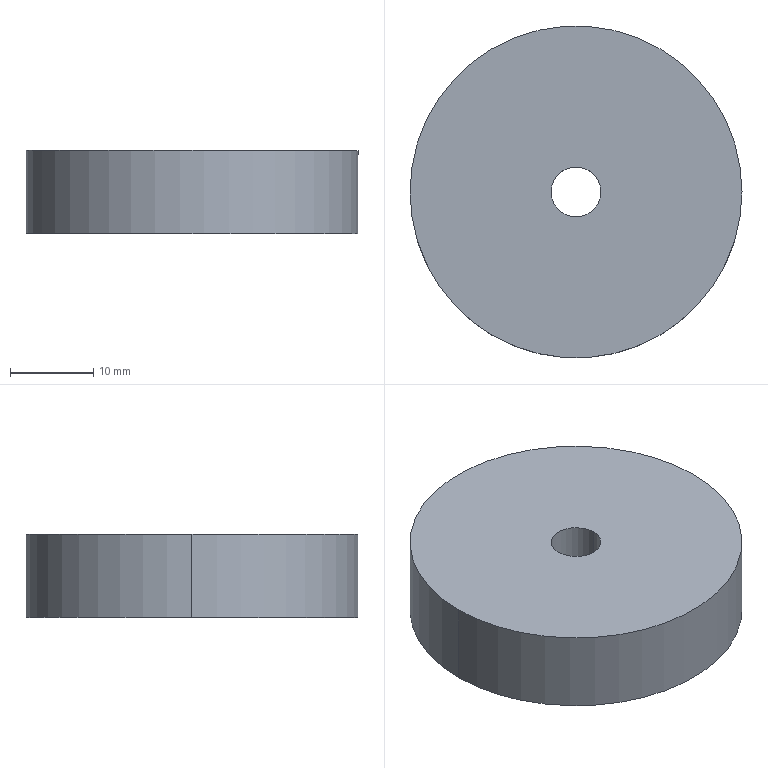Part | SolidWorks | features Revolution 1 | 1 solid | 6 faces | box 40 x 40 x 10 mm | volume 12284 mm3 | cylinder 4 | plane 2 | commonest cylinder face diameters 6 x2 40 x2
STEP:
#1=CARTESIAN_POINT('',(20.,0.,-10.));
#2=VERTEX_POINT('',#1);
#3=CARTESIAN_POINT('',(-20.,0.,-10.));
#4=VERTEX_POINT('',#3);
#5=CARTESIAN_POINT('',(0.,0.,-10.));
#6=DIRECTION('',(0.,0.,1.));
#7=DIRECTION('',(1.,0.,0.));
#8=AXIS2_PLACEMENT_3D('',#5,#6,#7);
#9=CIRCLE('',#8,20.);
#10=EDGE_CURVE('',#2,#4,#9,.T.);
#11=ORIENTED_EDGE('',*,*,#10,.T.);
#12=CARTESIAN_POINT('',(-20.,0.,0.));
#13=VERTEX_POINT('',#12);
#14=CARTESIAN_POINT('',(-20.,0.,129.063));
#15=DIRECTION('',(0.,0.,1.));
#16=VECTOR('',#15,1000.);
#17=LINE('',#14,#16);
#18=EDGE_CURVE('',#4,#13,#17,.T.);
#19=ORIENTED_EDGE('',*,*,#18,.T.);
#20=CARTESIAN_POINT('',(20.,0.,0.));
#21=VERTEX_POINT('',#20);
#22=CARTESIAN_POINT('',(0.,0.,0.));
#23=DIRECTION('',(0.,0.,1.));
#24=DIRECTION('',(1.,0.,0.));
#25=AXIS2_PLACEMENT_3D('',#22,#23,#24);
#26=CIRCLE('',#25,20.);
#27=EDGE_CURVE('',#21,#13,#26,.T.);
#28=ORIENTED_EDGE('',*,*,#27,.F.);
#29=CARTESIAN_POINT('',(20.,0.,129.063));
#30=DIRECTION('',(0.,0.,1.));
#31=VECTOR('',#30,1000.);
#32=LINE('',#29,#31);
#33=EDGE_CURVE('',#2,#21,#32,.T.);
#34=ORIENTED_EDGE('',*,*,#33,.F.);
#35=EDGE_LOOP('',(#11,#19,#28,#34));
#36=FACE_OUTER_BOUND('',#35,.T.);
#37=CARTESIAN_POINT('',(0.,0.,129.063));
#38=DIRECTION('',(0.,0.,1.));
#39=DIRECTION('',(1.,0.,0.));
#40=AXIS2_PLACEMENT_3D('',#37,#38,#39);
#41=CYLINDRICAL_SURFACE('',#40,20.);
#42=ADVANCED_FACE('',(#36),#41,.T.);
#43=CARTESIAN_POINT('',(-3.,0.,-10.));
#44=VERTEX_POINT('',#43);
#45=CARTESIAN_POINT('',(3.,0.,-10.));
#46=VERTEX_POINT('',#45);
#47=CARTESIAN_POINT('',(0.,0.,-10.));
#48=DIRECTION('',(0.,0.,1.));
#49=DIRECTION('',(1.,0.,0.));
#50=AXIS2_PLACEMENT_3D('',#47,#48,#49);
#51=CIRCLE('',#50,3.);
#52=EDGE_CURVE('',#44,#46,#51,.T.);
#53=ORIENTED_EDGE('',*,*,#52,.F.);
#54=CARTESIAN_POINT('',(-3.,0.,0.));
#55=VERTEX_POINT('',#54);
#56=CARTESIAN_POINT('',(-3.,0.,129.063));
#57=DIRECTION('',(0.,0.,1.));
#58=VECTOR('',#57,1000.);
#59=LINE('',#56,#58);
#60=EDGE_CURVE('',#44,#55,#59,.T.);
#61=ORIENTED_EDGE('',*,*,#60,.T.);
#62=CARTESIAN_POINT('',(3.,0.,0.));
#63=VERTEX_POINT('',#62);
#64=CARTESIAN_POINT('',(0.,0.,0.));
#65=DIRECTION('',(0.,0.,1.));
#66=DIRECTION('',(1.,0.,0.));
#67=AXIS2_PLACEMENT_3D('',#64,#65,#66);
#68=CIRCLE('',#67,3.);
#69=EDGE_CURVE('',#55,#63,#68,.T.);
#70=ORIENTED_EDGE('',*,*,#69,.T.);
#71=CARTESIAN_POINT('',(3.,0.,129.063));
#72=DIRECTION('',(0.,0.,1.));
#73=VECTOR('',#72,1000.);
#74=LINE('',#71,#73);
#75=EDGE_CURVE('',#46,#63,#74,.T.);
#76=ORIENTED_EDGE('',*,*,#75,.F.);
#77=EDGE_LOOP('',(#53,#61,#70,#76));
#78=FACE_OUTER_BOUND('',#77,.T.);
#79=CARTESIAN_POINT('',(0.,0.,129.063));
#80=DIRECTION('',(0.,0.,1.));
#81=DIRECTION('',(1.,0.,0.));
#82=AXIS2_PLACEMENT_3D('',#79,#80,#81);
#83=CYLINDRICAL_SURFACE('',#82,3.);
#84=ADVANCED_FACE('',(#78),#83,.F.);
#85=ORIENTED_EDGE('',*,*,#60,.F.);
#86=CARTESIAN_POINT('',(0.,0.,-10.));
#87=DIRECTION('',(0.,0.,1.));
#88=DIRECTION('',(1.,0.,0.));
#89=AXIS2_PLACEMENT_3D('',#86,#87,#88);
#90=CIRCLE('',#89,3.);
#91=EDGE_CURVE('',#46,#44,#90,.T.);
#92=ORIENTED_EDGE('',*,*,#91,.F.);
#93=ORIENTED_EDGE('',*,*,#75,.T.);
#94=CARTESIAN_POINT('',(0.,0.,0.));
#95=DIRECTION('',(0.,0.,1.));
#96=DIRECTION('',(1.,0.,0.));
#97=AXIS2_PLACEMENT_3D('',#94,#95,#96);
#98=CIRCLE('',#97,3.);
#99=EDGE_CURVE('',#63,#55,#98,.T.);
#100=ORIENTED_EDGE('',*,*,#99,.T.);
#101=EDGE_LOOP('',(#85,#92,#93,#100));
#102=FACE_OUTER_BOUND('',#101,.T.);
#103=CARTESIAN_POINT('',(0.,0.,129.063));
#104=DIRECTION('',(0.,0.,1.));
#105=DIRECTION('',(1.,0.,0.));
#106=AXIS2_PLACEMENT_3D('',#103,#104,#105);
#107=CYLINDRICAL_SURFACE('',#106,3.);
#108=ADVANCED_FACE('',(#102),#107,.F.);
#109=ORIENTED_EDGE('',*,*,#99,.F.);
#110=ORIENTED_EDGE('',*,*,#69,.F.);
#111=EDGE_LOOP('',(#109,#110));
#112=FACE_BOUND('',#111,.T.);
#113=ORIENTED_EDGE('',*,*,#27,.T.);
#114=CARTESIAN_POINT('',(0.,0.,0.));
#115=DIRECTION('',(0.,0.,1.));
#116=DIRECTION('',(1.,0.,0.));
#117=AXIS2_PLACEMENT_3D('',#114,#115,#116);
#118=CIRCLE('',#117,20.);
#119=EDGE_CURVE('',#13,#21,#118,.T.);
#120=ORIENTED_EDGE('',*,*,#119,.T.);
#121=EDGE_LOOP('',(#113,#120));
#122=FACE_OUTER_BOUND('',#121,.T.);
#123=CARTESIAN_POINT('',(-3.,0.,0.));
#124=DIRECTION('',(0.,0.,-1.));
#125=DIRECTION('',(-1.,0.,0.));
#126=AXIS2_PLACEMENT_3D('',#123,#124,#125);
#127=PLANE('',#126);
#128=ADVANCED_FACE('',(#112,#122),#127,.F.);
#129=ORIENTED_EDGE('',*,*,#18,.F.);
#130=CARTESIAN_POINT('',(0.,0.,-10.));
#131=DIRECTION('',(0.,0.,1.));
#132=DIRECTION('',(1.,0.,0.));
#133=AXIS2_PLACEMENT_3D('',#130,#131,#132);
#134=CIRCLE('',#133,20.);
#135=EDGE_CURVE('',#4,#2,#134,.T.);
#136=ORIENTED_EDGE('',*,*,#135,.T.);
#137=ORIENTED_EDGE('',*,*,#33,.T.);
#138=ORIENTED_EDGE('',*,*,#119,.F.);
#139=EDGE_LOOP('',(#129,#136,#137,#138));
#140=FACE_OUTER_BOUND('',#139,.T.);
#141=CARTESIAN_POINT('',(0.,0.,129.063));
#142=DIRECTION('',(0.,0.,1.));
#143=DIRECTION('',(1.,0.,0.));
#144=AXIS2_PLACEMENT_3D('',#141,#142,#143);
#145=CYLINDRICAL_SURFACE('',#144,20.);
#146=ADVANCED_FACE('',(#140),#145,.T.);
#147=ORIENTED_EDGE('',*,*,#10,.F.);
#148=ORIENTED_EDGE('',*,*,#135,.F.);
#149=EDGE_LOOP('',(#147,#148));
#150=FACE_OUTER_BOUND('',#149,.T.);
#151=ORIENTED_EDGE('',*,*,#91,.T.);
#152=ORIENTED_EDGE('',*,*,#52,.T.);
#153=EDGE_LOOP('',(#151,#152));
#154=FACE_BOUND('',#153,.T.);
#155=CARTESIAN_POINT('',(-20.,0.,-10.));
#156=DIRECTION('',(0.,0.,1.));
#157=DIRECTION('',(1.,0.,0.));
#158=AXIS2_PLACEMENT_3D('',#155,#156,#157);
#159=PLANE('',#158);
#160=ADVANCED_FACE('',(#150,#154),#159,.F.);
#161=CLOSED_SHELL('',(#42,#84,#108,#128,#146,#160));
#162=MANIFOLD_SOLID_BREP('',#161);
#163=CARTESIAN_POINT('',(0.,0.,0.));
#164=DIRECTION('',(0.,0.,1.));
#165=DIRECTION('',(1.,0.,0.));
#166=AXIS2_PLACEMENT_3D('',#163,#164,#165);
#167=(LENGTH_UNIT()NAMED_UNIT(*)SI_UNIT(.MILLI.,.METRE.));
#168=UNCERTAINTY_MEASURE_WITH_UNIT(LENGTH_MEASURE(0.00001),#167,'','');
#169=(NAMED_UNIT(*)PLANE_ANGLE_UNIT()SI_UNIT($,.RADIAN.));
#170=(NAMED_UNIT(*)SI_UNIT($,.STERADIAN.)SOLID_ANGLE_UNIT());
#171=(GEOMETRIC_REPRESENTATION_CONTEXT(3)GLOBAL_UNCERTAINTY_ASSIGNED_CONTEXT((#168))GLOBAL_UNIT_ASSIGNED_CONTEXT((#167,#169,#170))REPRESENTATION_CONTEXT('',''));
#172=ADVANCED_BREP_SHAPE_REPRESENTATION('',(#162,#166),#171);